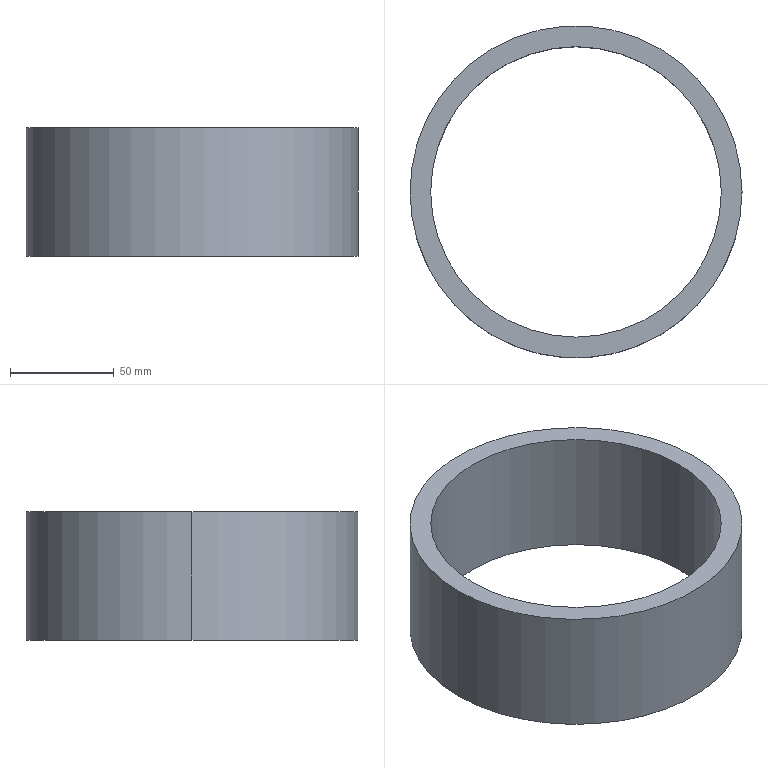Part | NX | features BREP 1, MOVE_FACE 1 | 1 solid | 6 faces | box 160 x 160 x 62 mm | volume 292168 mm3 | cylinder 4 | plane 2 | commonest cylinder face diameters 140 x2 160 x2
STEP:
#1=CARTESIAN_POINT('',(-70.,0.,-14.));
#2=VERTEX_POINT('',#1);
#3=CARTESIAN_POINT('',(70.,0.,-14.));
#4=VERTEX_POINT('',#3);
#5=CARTESIAN_POINT('',(0.,0.,-14.));
#6=DIRECTION('',(0.,0.,1.));
#7=DIRECTION('',(1.,0.,0.));
#8=AXIS2_PLACEMENT_3D('',#5,#6,#7);
#9=CIRCLE('',#8,70.);
#10=EDGE_CURVE('',#2,#4,#9,.T.);
#11=ORIENTED_EDGE('',*,*,#10,.T.);
#12=CARTESIAN_POINT('',(70.,0.,-76.));
#13=VERTEX_POINT('',#12);
#14=CARTESIAN_POINT('',(70.,0.,76.));
#15=DIRECTION('',(0.,0.,-1.));
#16=VECTOR('',#15,1000.);
#17=LINE('',#14,#16);
#18=EDGE_CURVE('',#13,#4,#17,.F.);
#19=ORIENTED_EDGE('',*,*,#18,.F.);
#20=CARTESIAN_POINT('',(-70.,0.,-76.));
#21=VERTEX_POINT('',#20);
#22=CARTESIAN_POINT('',(0.,0.,-76.));
#23=DIRECTION('',(0.,0.,1.));
#24=DIRECTION('',(1.,0.,0.));
#25=AXIS2_PLACEMENT_3D('',#22,#23,#24);
#26=CIRCLE('',#25,70.);
#27=EDGE_CURVE('',#21,#13,#26,.T.);
#28=ORIENTED_EDGE('',*,*,#27,.F.);
#29=CARTESIAN_POINT('',(-70.,0.,76.));
#30=DIRECTION('',(0.,0.,-1.));
#31=VECTOR('',#30,1000.);
#32=LINE('',#29,#31);
#33=EDGE_CURVE('',#21,#2,#32,.F.);
#34=ORIENTED_EDGE('',*,*,#33,.T.);
#35=EDGE_LOOP('',(#11,#19,#28,#34));
#36=FACE_BOUND('',#35,.T.);
#37=CARTESIAN_POINT('',(0.,0.,76.));
#38=DIRECTION('',(0.,0.,-1.));
#39=DIRECTION('',(1.,0.,0.));
#40=AXIS2_PLACEMENT_3D('',#37,#38,#39);
#41=CYLINDRICAL_SURFACE('',#40,70.);
#42=ADVANCED_FACE('',(#36),#41,.F.);
#43=CARTESIAN_POINT('',(80.,0.,-14.));
#44=VERTEX_POINT('',#43);
#45=CARTESIAN_POINT('',(-80.,0.,-14.));
#46=VERTEX_POINT('',#45);
#47=CARTESIAN_POINT('',(0.,0.,-14.));
#48=DIRECTION('',(0.,0.,1.));
#49=DIRECTION('',(1.,0.,0.));
#50=AXIS2_PLACEMENT_3D('',#47,#48,#49);
#51=CIRCLE('',#50,80.);
#52=EDGE_CURVE('',#44,#46,#51,.T.);
#53=ORIENTED_EDGE('',*,*,#52,.F.);
#54=CARTESIAN_POINT('',(80.,0.,-76.));
#55=VERTEX_POINT('',#54);
#56=CARTESIAN_POINT('',(80.,0.,76.));
#57=DIRECTION('',(0.,0.,-1.));
#58=VECTOR('',#57,1000.);
#59=LINE('',#56,#58);
#60=EDGE_CURVE('',#55,#44,#59,.F.);
#61=ORIENTED_EDGE('',*,*,#60,.F.);
#62=CARTESIAN_POINT('',(-80.,0.,-76.));
#63=VERTEX_POINT('',#62);
#64=CARTESIAN_POINT('',(0.,0.,-76.));
#65=DIRECTION('',(0.,0.,1.));
#66=DIRECTION('',(1.,0.,0.));
#67=AXIS2_PLACEMENT_3D('',#64,#65,#66);
#68=CIRCLE('',#67,80.);
#69=EDGE_CURVE('',#55,#63,#68,.T.);
#70=ORIENTED_EDGE('',*,*,#69,.T.);
#71=CARTESIAN_POINT('',(-80.,0.,76.));
#72=DIRECTION('',(0.,0.,-1.));
#73=VECTOR('',#72,1000.);
#74=LINE('',#71,#73);
#75=EDGE_CURVE('',#63,#46,#74,.F.);
#76=ORIENTED_EDGE('',*,*,#75,.T.);
#77=EDGE_LOOP('',(#53,#61,#70,#76));
#78=FACE_BOUND('',#77,.T.);
#79=CARTESIAN_POINT('',(0.,0.,76.));
#80=DIRECTION('',(0.,0.,-1.));
#81=DIRECTION('',(1.,0.,0.));
#82=AXIS2_PLACEMENT_3D('',#79,#80,#81);
#83=CYLINDRICAL_SURFACE('',#82,80.);
#84=ADVANCED_FACE('',(#78),#83,.T.);
#85=CARTESIAN_POINT('',(0.,0.,-14.));
#86=DIRECTION('',(0.,0.,1.));
#87=DIRECTION('',(1.,0.,0.));
#88=AXIS2_PLACEMENT_3D('',#85,#86,#87);
#89=CIRCLE('',#88,80.);
#90=EDGE_CURVE('',#46,#44,#89,.T.);
#91=ORIENTED_EDGE('',*,*,#90,.T.);
#92=ORIENTED_EDGE('',*,*,#52,.T.);
#93=EDGE_LOOP('',(#91,#92));
#94=FACE_BOUND('',#93,.T.);
#95=ORIENTED_EDGE('',*,*,#10,.F.);
#96=CARTESIAN_POINT('',(0.,0.,-14.));
#97=DIRECTION('',(0.,0.,1.));
#98=DIRECTION('',(1.,0.,0.));
#99=AXIS2_PLACEMENT_3D('',#96,#97,#98);
#100=CIRCLE('',#99,70.);
#101=EDGE_CURVE('',#4,#2,#100,.T.);
#102=ORIENTED_EDGE('',*,*,#101,.F.);
#103=EDGE_LOOP('',(#95,#102));
#104=FACE_BOUND('',#103,.T.);
#105=CARTESIAN_POINT('',(0.,0.,-14.));
#106=DIRECTION('',(0.,0.,1.));
#107=DIRECTION('',(-1.,0.,0.));
#108=AXIS2_PLACEMENT_3D('',#105,#106,#107);
#109=PLANE('',#108);
#110=ADVANCED_FACE('',(#94,#104),#109,.T.);
#111=CARTESIAN_POINT('',(0.,0.,-76.));
#112=DIRECTION('',(0.,0.,1.));
#113=DIRECTION('',(1.,0.,0.));
#114=AXIS2_PLACEMENT_3D('',#111,#112,#113);
#115=CIRCLE('',#114,80.);
#116=EDGE_CURVE('',#63,#55,#115,.T.);
#117=ORIENTED_EDGE('',*,*,#116,.F.);
#118=ORIENTED_EDGE('',*,*,#69,.F.);
#119=EDGE_LOOP('',(#117,#118));
#120=FACE_BOUND('',#119,.T.);
#121=ORIENTED_EDGE('',*,*,#27,.T.);
#122=CARTESIAN_POINT('',(0.,0.,-76.));
#123=DIRECTION('',(0.,0.,1.));
#124=DIRECTION('',(1.,0.,0.));
#125=AXIS2_PLACEMENT_3D('',#122,#123,#124);
#126=CIRCLE('',#125,70.);
#127=EDGE_CURVE('',#13,#21,#126,.T.);
#128=ORIENTED_EDGE('',*,*,#127,.T.);
#129=EDGE_LOOP('',(#121,#128));
#130=FACE_BOUND('',#129,.T.);
#131=CARTESIAN_POINT('',(0.,0.,-76.));
#132=DIRECTION('',(0.,0.,1.));
#133=DIRECTION('',(-1.,0.,0.));
#134=AXIS2_PLACEMENT_3D('',#131,#132,#133);
#135=PLANE('',#134);
#136=ADVANCED_FACE('',(#120,#130),#135,.F.);
#137=ORIENTED_EDGE('',*,*,#60,.T.);
#138=ORIENTED_EDGE('',*,*,#90,.F.);
#139=ORIENTED_EDGE('',*,*,#75,.F.);
#140=ORIENTED_EDGE('',*,*,#116,.T.);
#141=EDGE_LOOP('',(#137,#138,#139,#140));
#142=FACE_BOUND('',#141,.T.);
#143=CARTESIAN_POINT('',(0.,0.,76.));
#144=DIRECTION('',(0.,0.,-1.));
#145=DIRECTION('',(1.,0.,0.));
#146=AXIS2_PLACEMENT_3D('',#143,#144,#145);
#147=CYLINDRICAL_SURFACE('',#146,80.);
#148=ADVANCED_FACE('',(#142),#147,.T.);
#149=ORIENTED_EDGE('',*,*,#18,.T.);
#150=ORIENTED_EDGE('',*,*,#101,.T.);
#151=ORIENTED_EDGE('',*,*,#33,.F.);
#152=ORIENTED_EDGE('',*,*,#127,.F.);
#153=EDGE_LOOP('',(#149,#150,#151,#152));
#154=FACE_BOUND('',#153,.T.);
#155=CARTESIAN_POINT('',(0.,0.,76.));
#156=DIRECTION('',(0.,0.,-1.));
#157=DIRECTION('',(1.,0.,0.));
#158=AXIS2_PLACEMENT_3D('',#155,#156,#157);
#159=CYLINDRICAL_SURFACE('',#158,70.);
#160=ADVANCED_FACE('',(#154),#159,.F.);
#161=CLOSED_SHELL('',(#42,#84,#110,#136,#148,#160));
#162=MANIFOLD_SOLID_BREP('',#161);
#163=(LENGTH_UNIT()NAMED_UNIT(*)SI_UNIT(.MILLI.,.METRE.));
#164=UNCERTAINTY_MEASURE_WITH_UNIT(LENGTH_MEASURE(0.00001),#163,'','');
#165=(NAMED_UNIT(*)PLANE_ANGLE_UNIT()SI_UNIT($,.RADIAN.));
#166=(NAMED_UNIT(*)SI_UNIT($,.STERADIAN.)SOLID_ANGLE_UNIT());
#167=(GEOMETRIC_REPRESENTATION_CONTEXT(3)GLOBAL_UNCERTAINTY_ASSIGNED_CONTEXT((#164))GLOBAL_UNIT_ASSIGNED_CONTEXT((#163,#165,#166))REPRESENTATION_CONTEXT('',''));
#168=ADVANCED_BREP_SHAPE_REPRESENTATION('',(#162),#167);